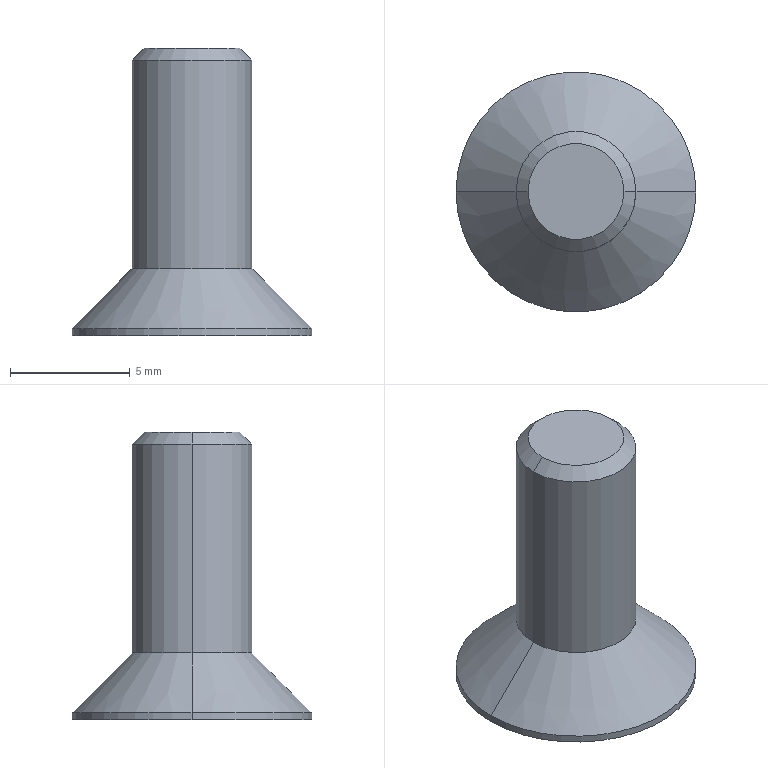Part | SolidWorks | features BaseBody 1 | 1 solid | 24 faces | box 10 x 10 x 12 mm | volume 284.359 mm3 | plane 14 | cone 6 | cylinder 4 | commonest cylinder face diameters 5 x2 10 x2
STEP:
#1=CARTESIAN_POINT('',(-2.5,0.,11.5));
#2=VERTEX_POINT('',#1);
#3=CARTESIAN_POINT('',(2.5,0.,11.5));
#4=VERTEX_POINT('',#3);
#5=CARTESIAN_POINT('',(0.,0.,11.5));
#6=DIRECTION('',(0.,0.,-1.));
#7=DIRECTION('',(-1.,0.,0.));
#8=AXIS2_PLACEMENT_3D('',#5,#6,#7);
#9=CIRCLE('',#8,2.5);
#10=EDGE_CURVE('',#2,#4,#9,.T.);
#11=ORIENTED_EDGE('',*,*,#10,.T.);
#12=CARTESIAN_POINT('',(2.5,0.,2.8));
#13=VERTEX_POINT('',#12);
#14=CARTESIAN_POINT('',(2.5,0.,12.));
#15=DIRECTION('',(0.,0.,-1.));
#16=VECTOR('',#15,1000.);
#17=LINE('',#14,#16);
#18=EDGE_CURVE('',#4,#13,#17,.T.);
#19=ORIENTED_EDGE('',*,*,#18,.T.);
#20=CARTESIAN_POINT('',(-2.5,0.,2.8));
#21=VERTEX_POINT('',#20);
#22=CARTESIAN_POINT('',(0.,0.,2.8));
#23=DIRECTION('',(0.,0.,1.));
#24=DIRECTION('',(-1.,0.,0.));
#25=AXIS2_PLACEMENT_3D('',#22,#23,#24);
#26=CIRCLE('',#25,2.5);
#27=EDGE_CURVE('',#13,#21,#26,.T.);
#28=ORIENTED_EDGE('',*,*,#27,.T.);
#29=CARTESIAN_POINT('',(-2.5,0.,12.));
#30=DIRECTION('',(0.,0.,-1.));
#31=VECTOR('',#30,1000.);
#32=LINE('',#29,#31);
#33=EDGE_CURVE('',#2,#21,#32,.T.);
#34=ORIENTED_EDGE('',*,*,#33,.F.);
#35=EDGE_LOOP('',(#11,#19,#28,#34));
#36=FACE_OUTER_BOUND('',#35,.T.);
#37=CARTESIAN_POINT('',(0.,0.,12.));
#38=DIRECTION('',(0.,0.,-1.));
#39=DIRECTION('',(-1.,0.,0.));
#40=AXIS2_PLACEMENT_3D('',#37,#38,#39);
#41=CYLINDRICAL_SURFACE('',#40,2.5);
#42=ADVANCED_FACE('',(#36),#41,.T.);
#43=ORIENTED_EDGE('',*,*,#27,.F.);
#44=CARTESIAN_POINT('',(5.,0.,0.3));
#45=VERTEX_POINT('',#44);
#46=CARTESIAN_POINT('',(5.,0.,0.3));
#47=DIRECTION('',(0.7071,0.,-0.7071));
#48=VECTOR('',#47,1000.);
#49=LINE('',#46,#48);
#50=EDGE_CURVE('',#13,#45,#49,.T.);
#51=ORIENTED_EDGE('',*,*,#50,.T.);
#52=CARTESIAN_POINT('',(-5.,0.,0.3));
#53=VERTEX_POINT('',#52);
#54=CARTESIAN_POINT('',(0.,0.,0.3));
#55=DIRECTION('',(0.,0.,1.));
#56=DIRECTION('',(-1.,0.,0.));
#57=AXIS2_PLACEMENT_3D('',#54,#55,#56);
#58=CIRCLE('',#57,5.);
#59=EDGE_CURVE('',#45,#53,#58,.T.);
#60=ORIENTED_EDGE('',*,*,#59,.T.);
#61=CARTESIAN_POINT('',(-5.,0.,0.3));
#62=DIRECTION('',(-0.7071,0.,-0.7071));
#63=VECTOR('',#62,1000.);
#64=LINE('',#61,#63);
#65=EDGE_CURVE('',#21,#53,#64,.T.);
#66=ORIENTED_EDGE('',*,*,#65,.F.);
#67=EDGE_LOOP('',(#43,#51,#60,#66));
#68=FACE_OUTER_BOUND('',#67,.T.);
#69=CARTESIAN_POINT('',(0.,0.,0.3));
#70=DIRECTION('',(0.,0.,-1.));
#71=DIRECTION('',(-1.,0.,0.));
#72=AXIS2_PLACEMENT_3D('',#69,#70,#71);
#73=CONICAL_SURFACE('',#72,5.,0.7854);
#74=ADVANCED_FACE('',(#68),#73,.T.);
#75=CARTESIAN_POINT('',(-2.,0.,12.));
#76=VERTEX_POINT('',#75);
#77=CARTESIAN_POINT('',(2.,0.,12.));
#78=VERTEX_POINT('',#77);
#79=CARTESIAN_POINT('',(0.,0.,12.));
#80=DIRECTION('',(0.,0.,-1.));
#81=DIRECTION('',(-1.,0.,0.));
#82=AXIS2_PLACEMENT_3D('',#79,#80,#81);
#83=CIRCLE('',#82,2.);
#84=EDGE_CURVE('',#76,#78,#83,.T.);
#85=ORIENTED_EDGE('',*,*,#84,.T.);
#86=CARTESIAN_POINT('',(2.5,0.,11.5));
#87=DIRECTION('',(0.7071,0.,-0.7071));
#88=VECTOR('',#87,1000.);
#89=LINE('',#86,#88);
#90=EDGE_CURVE('',#78,#4,#89,.T.);
#91=ORIENTED_EDGE('',*,*,#90,.T.);
#92=ORIENTED_EDGE('',*,*,#10,.F.);
#93=CARTESIAN_POINT('',(-2.5,0.,11.5));
#94=DIRECTION('',(-0.7071,0.,-0.7071));
#95=VECTOR('',#94,1000.);
#96=LINE('',#93,#95);
#97=EDGE_CURVE('',#76,#2,#96,.T.);
#98=ORIENTED_EDGE('',*,*,#97,.F.);
#99=EDGE_LOOP('',(#85,#91,#92,#98));
#100=FACE_OUTER_BOUND('',#99,.T.);
#101=CARTESIAN_POINT('',(0.,0.,11.5));
#102=DIRECTION('',(0.,0.,-1.));
#103=DIRECTION('',(-1.,0.,0.));
#104=AXIS2_PLACEMENT_3D('',#101,#102,#103);
#105=CONICAL_SURFACE('',#104,2.5,0.7854);
#106=ADVANCED_FACE('',(#100),#105,.T.);
#107=ORIENTED_EDGE('',*,*,#59,.F.);
#108=CARTESIAN_POINT('',(5.,0.,0.));
#109=VERTEX_POINT('',#108);
#110=CARTESIAN_POINT('',(5.,0.,2.8));
#111=DIRECTION('',(0.,0.,-1.));
#112=VECTOR('',#111,1000.);
#113=LINE('',#110,#112);
#114=EDGE_CURVE('',#45,#109,#113,.T.);
#115=ORIENTED_EDGE('',*,*,#114,.T.);
#116=CARTESIAN_POINT('',(-5.,0.,0.));
#117=VERTEX_POINT('',#116);
#118=CARTESIAN_POINT('',(0.,0.,0.));
#119=DIRECTION('',(0.,0.,1.));
#120=DIRECTION('',(-1.,0.,0.));
#121=AXIS2_PLACEMENT_3D('',#118,#119,#120);
#122=CIRCLE('',#121,5.);
#123=EDGE_CURVE('',#109,#117,#122,.T.);
#124=ORIENTED_EDGE('',*,*,#123,.T.);
#125=CARTESIAN_POINT('',(-5.,0.,2.8));
#126=DIRECTION('',(0.,0.,-1.));
#127=VECTOR('',#126,1000.);
#128=LINE('',#125,#127);
#129=EDGE_CURVE('',#53,#117,#128,.T.);
#130=ORIENTED_EDGE('',*,*,#129,.F.);
#131=EDGE_LOOP('',(#107,#115,#124,#130));
#132=FACE_OUTER_BOUND('',#131,.T.);
#133=CARTESIAN_POINT('',(0.,0.,2.8));
#134=DIRECTION('',(0.,0.,-1.));
#135=DIRECTION('',(-1.,0.,0.));
#136=AXIS2_PLACEMENT_3D('',#133,#134,#135);
#137=CYLINDRICAL_SURFACE('',#136,5.);
#138=ADVANCED_FACE('',(#132),#137,.T.);
#139=CARTESIAN_POINT('',(0.,0.,3.155));
#140=VERTEX_POINT('',#139);
#141=CARTESIAN_POINT('',(-2.,0.,2.));
#142=VERTEX_POINT('',#141);
#143=CARTESIAN_POINT('',(-2.,0.,2.));
#144=DIRECTION('',(-0.866,0.,-0.5));
#145=VECTOR('',#144,1000.);
#146=LINE('',#143,#145);
#147=EDGE_CURVE('',#140,#142,#146,.T.);
#148=ORIENTED_EDGE('',*,*,#147,.F.);
#149=CARTESIAN_POINT('',(2.,0.,2.));
#150=VERTEX_POINT('',#149);
#151=CARTESIAN_POINT('',(2.,0.,2.));
#152=DIRECTION('',(0.866,0.,-0.5));
#153=VECTOR('',#152,1000.);
#154=LINE('',#151,#153);
#155=EDGE_CURVE('',#140,#150,#154,.T.);
#156=ORIENTED_EDGE('',*,*,#155,.T.);
#157=CARTESIAN_POINT('',(1.732,-1.,2.));
#158=VERTEX_POINT('',#157);
#159=CARTESIAN_POINT('',(0.,0.,2.));
#160=DIRECTION('',(0.,0.,1.));
#161=DIRECTION('',(-1.,0.,0.));
#162=AXIS2_PLACEMENT_3D('',#159,#160,#161);
#163=CIRCLE('',#162,2.);
#164=EDGE_CURVE('',#158,#150,#163,.T.);
#165=ORIENTED_EDGE('',*,*,#164,.F.);
#166=CARTESIAN_POINT('',(0.,-2.,2.));
#167=VERTEX_POINT('',#166);
#168=CARTESIAN_POINT('',(0.,0.,2.));
#169=DIRECTION('',(0.,0.,1.));
#170=DIRECTION('',(-1.,0.,0.));
#171=AXIS2_PLACEMENT_3D('',#168,#169,#170);
#172=CIRCLE('',#171,2.);
#173=EDGE_CURVE('',#167,#158,#172,.T.);
#174=ORIENTED_EDGE('',*,*,#173,.F.);
#175=CARTESIAN_POINT('',(-1.732,-1.,2.));
#176=VERTEX_POINT('',#175);
#177=CARTESIAN_POINT('',(0.,0.,2.));
#178=DIRECTION('',(0.,0.,1.));
#179=DIRECTION('',(-1.,0.,0.));
#180=AXIS2_PLACEMENT_3D('',#177,#178,#179);
#181=CIRCLE('',#180,2.);
#182=EDGE_CURVE('',#176,#167,#181,.T.);
#183=ORIENTED_EDGE('',*,*,#182,.F.);
#184=CARTESIAN_POINT('',(0.,0.,2.));
#185=DIRECTION('',(0.,0.,1.));
#186=DIRECTION('',(-1.,0.,0.));
#187=AXIS2_PLACEMENT_3D('',#184,#185,#186);
#188=CIRCLE('',#187,2.);
#189=EDGE_CURVE('',#142,#176,#188,.T.);
#190=ORIENTED_EDGE('',*,*,#189,.F.);
#191=EDGE_LOOP('',(#148,#156,#165,#174,#183,#190));
#192=FACE_OUTER_BOUND('',#191,.T.);
#193=CARTESIAN_POINT('',(0.,0.,2.));
#194=DIRECTION('',(0.,0.,-1.));
#195=DIRECTION('',(-1.,0.,0.));
#196=AXIS2_PLACEMENT_3D('',#193,#194,#195);
#197=CONICAL_SURFACE('',#196,2.,1.047);
#198=ADVANCED_FACE('',(#192),#197,.F.);
#199=ORIENTED_EDGE('',*,*,#18,.F.);
#200=CARTESIAN_POINT('',(0.,0.,11.5));
#201=DIRECTION('',(0.,0.,-1.));
#202=DIRECTION('',(-1.,0.,0.));
#203=AXIS2_PLACEMENT_3D('',#200,#201,#202);
#204=CIRCLE('',#203,2.5);
#205=EDGE_CURVE('',#4,#2,#204,.T.);
#206=ORIENTED_EDGE('',*,*,#205,.T.);
#207=ORIENTED_EDGE('',*,*,#33,.T.);
#208=CARTESIAN_POINT('',(0.,0.,2.8));
#209=DIRECTION('',(0.,0.,1.));
#210=DIRECTION('',(-1.,0.,0.));
#211=AXIS2_PLACEMENT_3D('',#208,#209,#210);
#212=CIRCLE('',#211,2.5);
#213=EDGE_CURVE('',#21,#13,#212,.T.);
#214=ORIENTED_EDGE('',*,*,#213,.T.);
#215=EDGE_LOOP('',(#199,#206,#207,#214));
#216=FACE_OUTER_BOUND('',#215,.T.);
#217=CARTESIAN_POINT('',(0.,0.,12.));
#218=DIRECTION('',(0.,0.,-1.));
#219=DIRECTION('',(-1.,0.,0.));
#220=AXIS2_PLACEMENT_3D('',#217,#218,#219);
#221=CYLINDRICAL_SURFACE('',#220,2.5);
#222=ADVANCED_FACE('',(#216),#221,.T.);
#223=ORIENTED_EDGE('',*,*,#50,.F.);
#224=ORIENTED_EDGE('',*,*,#213,.F.);
#225=ORIENTED_EDGE('',*,*,#65,.T.);
#226=CARTESIAN_POINT('',(0.,0.,0.3));
#227=DIRECTION('',(0.,0.,1.));
#228=DIRECTION('',(-1.,0.,0.));
#229=AXIS2_PLACEMENT_3D('',#226,#227,#228);
#230=CIRCLE('',#229,5.);
#231=EDGE_CURVE('',#53,#45,#230,.T.);
#232=ORIENTED_EDGE('',*,*,#231,.T.);
#233=EDGE_LOOP('',(#223,#224,#225,#232));
#234=FACE_OUTER_BOUND('',#233,.T.);
#235=CARTESIAN_POINT('',(0.,0.,0.3));
#236=DIRECTION('',(0.,0.,-1.));
#237=DIRECTION('',(-1.,0.,0.));
#238=AXIS2_PLACEMENT_3D('',#235,#236,#237);
#239=CONICAL_SURFACE('',#238,5.,0.7854);
#240=ADVANCED_FACE('',(#234),#239,.T.);
#241=ORIENTED_EDGE('',*,*,#90,.F.);
#242=CARTESIAN_POINT('',(0.,0.,12.));
#243=DIRECTION('',(0.,0.,-1.));
#244=DIRECTION('',(-1.,0.,0.));
#245=AXIS2_PLACEMENT_3D('',#242,#243,#244);
#246=CIRCLE('',#245,2.);
#247=EDGE_CURVE('',#78,#76,#246,.T.);
#248=ORIENTED_EDGE('',*,*,#247,.T.);
#249=ORIENTED_EDGE('',*,*,#97,.T.);
#250=ORIENTED_EDGE('',*,*,#205,.F.);
#251=EDGE_LOOP('',(#241,#248,#249,#250));
#252=FACE_OUTER_BOUND('',#251,.T.);
#253=CARTESIAN_POINT('',(0.,0.,11.5));
#254=DIRECTION('',(0.,0.,-1.));
#255=DIRECTION('',(-1.,0.,0.));
#256=AXIS2_PLACEMENT_3D('',#253,#254,#255);
#257=CONICAL_SURFACE('',#256,2.5,0.7854);
#258=ADVANCED_FACE('',(#252),#257,.T.);
#259=ORIENTED_EDGE('',*,*,#114,.F.);
#260=ORIENTED_EDGE('',*,*,#231,.F.);
#261=ORIENTED_EDGE('',*,*,#129,.T.);
#262=CARTESIAN_POINT('',(0.,0.,0.));
#263=DIRECTION('',(0.,0.,1.));
#264=DIRECTION('',(-1.,0.,0.));
#265=AXIS2_PLACEMENT_3D('',#262,#263,#264);
#266=CIRCLE('',#265,5.);
#267=EDGE_CURVE('',#117,#109,#266,.T.);
#268=ORIENTED_EDGE('',*,*,#267,.T.);
#269=EDGE_LOOP('',(#259,#260,#261,#268));
#270=FACE_OUTER_BOUND('',#269,.T.);
#271=CARTESIAN_POINT('',(0.,0.,2.8));
#272=DIRECTION('',(0.,0.,-1.));
#273=DIRECTION('',(-1.,0.,0.));
#274=AXIS2_PLACEMENT_3D('',#271,#272,#273);
#275=CYLINDRICAL_SURFACE('',#274,5.);
#276=ADVANCED_FACE('',(#270),#275,.T.);
#277=ORIENTED_EDGE('',*,*,#84,.F.);
#278=ORIENTED_EDGE('',*,*,#247,.F.);
#279=EDGE_LOOP('',(#277,#278));
#280=FACE_OUTER_BOUND('',#279,.T.);
#281=CARTESIAN_POINT('',(0.,0.,12.));
#282=DIRECTION('',(0.,0.,1.));
#283=DIRECTION('',(1.,0.,0.));
#284=AXIS2_PLACEMENT_3D('',#281,#282,#283);
#285=PLANE('',#284);
#286=ADVANCED_FACE('',(#280),#285,.T.);
#287=ORIENTED_EDGE('',*,*,#267,.F.);
#288=ORIENTED_EDGE('',*,*,#123,.F.);
#289=EDGE_LOOP('',(#287,#288));
#290=FACE_OUTER_BOUND('',#289,.T.);
#291=CARTESIAN_POINT('',(-2.309,0.,0.));
#292=VERTEX_POINT('',#291);
#293=CARTESIAN_POINT('',(-1.155,2.,0.));
#294=VERTEX_POINT('',#293);
#295=CARTESIAN_POINT('',(-2.309,0.,0.));
#296=DIRECTION('',(0.5,0.866,0.));
#297=VECTOR('',#296,1000.);
#298=LINE('',#295,#297);
#299=EDGE_CURVE('',#292,#294,#298,.T.);
#300=ORIENTED_EDGE('',*,*,#299,.F.);
#301=CARTESIAN_POINT('',(-1.155,-2.,0.));
#302=VERTEX_POINT('',#301);
#303=CARTESIAN_POINT('',(-1.155,-2.,0.));
#304=DIRECTION('',(-0.5,0.866,0.));
#305=VECTOR('',#304,1000.);
#306=LINE('',#303,#305);
#307=EDGE_CURVE('',#302,#292,#306,.T.);
#308=ORIENTED_EDGE('',*,*,#307,.F.);
#309=CARTESIAN_POINT('',(1.155,-2.,0.));
#310=VERTEX_POINT('',#309);
#311=CARTESIAN_POINT('',(0.,-2.,0.));
#312=DIRECTION('',(-1.,0.,0.));
#313=VECTOR('',#312,1000.);
#314=LINE('',#311,#313);
#315=EDGE_CURVE('',#310,#302,#314,.T.);
#316=ORIENTED_EDGE('',*,*,#315,.F.);
#317=CARTESIAN_POINT('',(2.309,0.,0.));
#318=VERTEX_POINT('',#317);
#319=CARTESIAN_POINT('',(2.309,0.,0.));
#320=DIRECTION('',(-0.5,-0.866,0.));
#321=VECTOR('',#320,1000.);
#322=LINE('',#319,#321);
#323=EDGE_CURVE('',#318,#310,#322,.T.);
#324=ORIENTED_EDGE('',*,*,#323,.F.);
#325=CARTESIAN_POINT('',(1.155,2.,0.));
#326=VERTEX_POINT('',#325);
#327=CARTESIAN_POINT('',(1.155,2.,0.));
#328=DIRECTION('',(0.5,-0.866,0.));
#329=VECTOR('',#328,1000.);
#330=LINE('',#327,#329);
#331=EDGE_CURVE('',#326,#318,#330,.T.);
#332=ORIENTED_EDGE('',*,*,#331,.F.);
#333=CARTESIAN_POINT('',(0.,2.,0.));
#334=DIRECTION('',(1.,0.,0.));
#335=VECTOR('',#334,1000.);
#336=LINE('',#333,#335);
#337=EDGE_CURVE('',#294,#326,#336,.T.);
#338=ORIENTED_EDGE('',*,*,#337,.F.);
#339=EDGE_LOOP('',(#300,#308,#316,#324,#332,#338));
#340=FACE_BOUND('',#339,.T.);
#341=CARTESIAN_POINT('',(0.,0.,0.));
#342=DIRECTION('',(0.,0.,1.));
#343=DIRECTION('',(1.,0.,0.));
#344=AXIS2_PLACEMENT_3D('',#341,#342,#343);
#345=PLANE('',#344);
#346=ADVANCED_FACE('',(#290,#340),#345,.F.);
#347=CARTESIAN_POINT('',(1.155,2.,2.));
#348=VERTEX_POINT('',#347);
#349=CARTESIAN_POINT('',(1.155,2.,2.));
#350=DIRECTION('',(0.,0.,-1.));
#351=VECTOR('',#350,1000.);
#352=LINE('',#349,#351);
#353=EDGE_CURVE('',#348,#326,#352,.T.);
#354=ORIENTED_EDGE('',*,*,#353,.F.);
#355=CARTESIAN_POINT('',(0.,2.,2.));
#356=VERTEX_POINT('',#355);
#357=CARTESIAN_POINT('',(0.,2.,2.));
#358=DIRECTION('',(1.,0.,0.));
#359=VECTOR('',#358,1000.);
#360=LINE('',#357,#359);
#361=EDGE_CURVE('',#356,#348,#360,.T.);
#362=ORIENTED_EDGE('',*,*,#361,.F.);
#363=CARTESIAN_POINT('',(-1.155,2.,2.));
#364=VERTEX_POINT('',#363);
#365=CARTESIAN_POINT('',(0.,2.,2.));
#366=DIRECTION('',(1.,0.,0.));
#367=VECTOR('',#366,1000.);
#368=LINE('',#365,#367);
#369=EDGE_CURVE('',#364,#356,#368,.T.);
#370=ORIENTED_EDGE('',*,*,#369,.F.);
#371=CARTESIAN_POINT('',(-1.155,2.,2.));
#372=DIRECTION('',(0.,0.,1.));
#373=VECTOR('',#372,1000.);
#374=LINE('',#371,#373);
#375=EDGE_CURVE('',#294,#364,#374,.T.);
#376=ORIENTED_EDGE('',*,*,#375,.F.);
#377=ORIENTED_EDGE('',*,*,#337,.T.);
#378=EDGE_LOOP('',(#354,#362,#370,#376,#377));
#379=FACE_OUTER_BOUND('',#378,.T.);
#380=CARTESIAN_POINT('',(-1.155,2.,2.));
#381=DIRECTION('',(0.,1.,0.));
#382=DIRECTION('',(0.,0.,1.));
#383=AXIS2_PLACEMENT_3D('',#380,#381,#382);
#384=PLANE('',#383);
#385=ADVANCED_FACE('',(#379),#384,.F.);
#386=ORIENTED_EDGE('',*,*,#375,.T.);
#387=CARTESIAN_POINT('',(-1.732,1.,2.));
#388=VERTEX_POINT('',#387);
#389=CARTESIAN_POINT('',(-1.732,1.,2.));
#390=DIRECTION('',(0.5,0.866,0.));
#391=VECTOR('',#390,1000.);
#392=LINE('',#389,#391);
#393=EDGE_CURVE('',#388,#364,#392,.T.);
#394=ORIENTED_EDGE('',*,*,#393,.F.);
#395=CARTESIAN_POINT('',(-2.309,0.,2.));
#396=VERTEX_POINT('',#395);
#397=CARTESIAN_POINT('',(-2.309,0.,2.));
#398=DIRECTION('',(0.5,0.866,0.));
#399=VECTOR('',#398,1000.);
#400=LINE('',#397,#399);
#401=EDGE_CURVE('',#396,#388,#400,.T.);
#402=ORIENTED_EDGE('',*,*,#401,.F.);
#403=CARTESIAN_POINT('',(-2.309,0.,2.));
#404=DIRECTION('',(0.,0.,1.));
#405=VECTOR('',#404,1000.);
#406=LINE('',#403,#405);
#407=EDGE_CURVE('',#292,#396,#406,.T.);
#408=ORIENTED_EDGE('',*,*,#407,.F.);
#409=ORIENTED_EDGE('',*,*,#299,.T.);
#410=EDGE_LOOP('',(#386,#394,#402,#408,#409));
#411=FACE_OUTER_BOUND('',#410,.T.);
#412=CARTESIAN_POINT('',(-2.309,0.,2.));
#413=DIRECTION('',(-0.866,0.5,0.));
#414=DIRECTION('',(-0.5,-0.866,0.));
#415=AXIS2_PLACEMENT_3D('',#412,#413,#414);
#416=PLANE('',#415);
#417=ADVANCED_FACE('',(#411),#416,.F.);
#418=ORIENTED_EDGE('',*,*,#407,.T.);
#419=CARTESIAN_POINT('',(-1.155,-2.,2.));
#420=DIRECTION('',(-0.5,0.866,0.));
#421=VECTOR('',#420,1000.);
#422=LINE('',#419,#421);
#423=EDGE_CURVE('',#176,#396,#422,.T.);
#424=ORIENTED_EDGE('',*,*,#423,.F.);
#425=CARTESIAN_POINT('',(-1.155,-2.,2.));
#426=VERTEX_POINT('',#425);
#427=CARTESIAN_POINT('',(-1.155,-2.,2.));
#428=DIRECTION('',(-0.5,0.866,0.));
#429=VECTOR('',#428,1000.);
#430=LINE('',#427,#429);
#431=EDGE_CURVE('',#426,#176,#430,.T.);
#432=ORIENTED_EDGE('',*,*,#431,.F.);
#433=CARTESIAN_POINT('',(-1.155,-2.,2.));
#434=DIRECTION('',(0.,0.,1.));
#435=VECTOR('',#434,1000.);
#436=LINE('',#433,#435);
#437=EDGE_CURVE('',#302,#426,#436,.T.);
#438=ORIENTED_EDGE('',*,*,#437,.F.);
#439=ORIENTED_EDGE('',*,*,#307,.T.);
#440=EDGE_LOOP('',(#418,#424,#432,#438,#439));
#441=FACE_OUTER_BOUND('',#440,.T.);
#442=CARTESIAN_POINT('',(-1.155,-2.,2.));
#443=DIRECTION('',(-0.866,-0.5,0.));
#444=DIRECTION('',(0.5,-0.866,0.));
#445=AXIS2_PLACEMENT_3D('',#442,#443,#444);
#446=PLANE('',#445);
#447=ADVANCED_FACE('',(#441),#446,.F.);
#448=ORIENTED_EDGE('',*,*,#437,.T.);
#449=CARTESIAN_POINT('',(0.,-2.,2.));
#450=DIRECTION('',(-1.,0.,0.));
#451=VECTOR('',#450,1000.);
#452=LINE('',#449,#451);
#453=EDGE_CURVE('',#167,#426,#452,.T.);
#454=ORIENTED_EDGE('',*,*,#453,.F.);
#455=CARTESIAN_POINT('',(1.155,-2.,2.));
#456=VERTEX_POINT('',#455);
#457=CARTESIAN_POINT('',(0.,-2.,2.));
#458=DIRECTION('',(-1.,0.,0.));
#459=VECTOR('',#458,1000.);
#460=LINE('',#457,#459);
#461=EDGE_CURVE('',#456,#167,#460,.T.);
#462=ORIENTED_EDGE('',*,*,#461,.F.);
#463=CARTESIAN_POINT('',(1.155,-2.,2.));
#464=DIRECTION('',(0.,0.,1.));
#465=VECTOR('',#464,1000.);
#466=LINE('',#463,#465);
#467=EDGE_CURVE('',#310,#456,#466,.T.);
#468=ORIENTED_EDGE('',*,*,#467,.F.);
#469=ORIENTED_EDGE('',*,*,#315,.T.);
#470=EDGE_LOOP('',(#448,#454,#462,#468,#469));
#471=FACE_OUTER_BOUND('',#470,.T.);
#472=CARTESIAN_POINT('',(1.155,-2.,2.));
#473=DIRECTION('',(0.,-1.,0.));
#474=DIRECTION('',(1.,0.,0.));
#475=AXIS2_PLACEMENT_3D('',#472,#473,#474);
#476=PLANE('',#475);
#477=ADVANCED_FACE('',(#471),#476,.F.);
#478=ORIENTED_EDGE('',*,*,#467,.T.);
#479=CARTESIAN_POINT('',(1.732,-1.,2.));
#480=DIRECTION('',(-0.5,-0.866,0.));
#481=VECTOR('',#480,1000.);
#482=LINE('',#479,#481);
#483=EDGE_CURVE('',#158,#456,#482,.T.);
#484=ORIENTED_EDGE('',*,*,#483,.F.);
#485=CARTESIAN_POINT('',(2.309,0.,2.));
#486=VERTEX_POINT('',#485);
#487=CARTESIAN_POINT('',(2.309,0.,2.));
#488=DIRECTION('',(-0.5,-0.866,0.));
#489=VECTOR('',#488,1000.);
#490=LINE('',#487,#489);
#491=EDGE_CURVE('',#486,#158,#490,.T.);
#492=ORIENTED_EDGE('',*,*,#491,.F.);
#493=CARTESIAN_POINT('',(2.309,0.,2.));
#494=DIRECTION('',(0.,0.,1.));
#495=VECTOR('',#494,1000.);
#496=LINE('',#493,#495);
#497=EDGE_CURVE('',#318,#486,#496,.T.);
#498=ORIENTED_EDGE('',*,*,#497,.F.);
#499=ORIENTED_EDGE('',*,*,#323,.T.);
#500=EDGE_LOOP('',(#478,#484,#492,#498,#499));
#501=FACE_OUTER_BOUND('',#500,.T.);
#502=CARTESIAN_POINT('',(2.309,0.,2.));
#503=DIRECTION('',(0.866,-0.5,0.));
#504=DIRECTION('',(0.5,0.866,0.));
#505=AXIS2_PLACEMENT_3D('',#502,#503,#504);
#506=PLANE('',#505);
#507=ADVANCED_FACE('',(#501),#506,.F.);
#508=ORIENTED_EDGE('',*,*,#497,.T.);
#509=CARTESIAN_POINT('',(1.732,1.,2.));
#510=VERTEX_POINT('',#509);
#511=CARTESIAN_POINT('',(1.155,2.,2.));
#512=DIRECTION('',(0.5,-0.866,0.));
#513=VECTOR('',#512,1000.);
#514=LINE('',#511,#513);
#515=EDGE_CURVE('',#510,#486,#514,.T.);
#516=ORIENTED_EDGE('',*,*,#515,.F.);
#517=CARTESIAN_POINT('',(1.155,2.,2.));
#518=DIRECTION('',(0.5,-0.866,0.));
#519=VECTOR('',#518,1000.);
#520=LINE('',#517,#519);
#521=EDGE_CURVE('',#348,#510,#520,.T.);
#522=ORIENTED_EDGE('',*,*,#521,.F.);
#523=ORIENTED_EDGE('',*,*,#353,.T.);
#524=ORIENTED_EDGE('',*,*,#331,.T.);
#525=EDGE_LOOP('',(#508,#516,#522,#523,#524));
#526=FACE_OUTER_BOUND('',#525,.T.);
#527=CARTESIAN_POINT('',(1.155,2.,2.));
#528=DIRECTION('',(0.866,0.5,0.));
#529=DIRECTION('',(-0.5,0.866,0.));
#530=AXIS2_PLACEMENT_3D('',#527,#528,#529);
#531=PLANE('',#530);
#532=ADVANCED_FACE('',(#526),#531,.F.);
#533=ORIENTED_EDGE('',*,*,#401,.T.);
#534=CARTESIAN_POINT('',(0.,0.,2.));
#535=DIRECTION('',(0.,0.,1.));
#536=DIRECTION('',(-1.,0.,0.));
#537=AXIS2_PLACEMENT_3D('',#534,#535,#536);
#538=CIRCLE('',#537,2.);
#539=EDGE_CURVE('',#388,#142,#538,.T.);
#540=ORIENTED_EDGE('',*,*,#539,.T.);
#541=ORIENTED_EDGE('',*,*,#189,.T.);
#542=ORIENTED_EDGE('',*,*,#423,.T.);
#543=EDGE_LOOP('',(#533,#540,#541,#542));
#544=FACE_OUTER_BOUND('',#543,.T.);
#545=CARTESIAN_POINT('',(0.,0.,2.));
#546=DIRECTION('',(0.,0.,-1.));
#547=DIRECTION('',(-1.,0.,0.));
#548=AXIS2_PLACEMENT_3D('',#545,#546,#547);
#549=PLANE('',#548);
#550=ADVANCED_FACE('',(#544),#549,.T.);
#551=ORIENTED_EDGE('',*,*,#491,.T.);
#552=ORIENTED_EDGE('',*,*,#164,.T.);
#553=CARTESIAN_POINT('',(0.,0.,2.));
#554=DIRECTION('',(0.,0.,1.));
#555=DIRECTION('',(-1.,0.,0.));
#556=AXIS2_PLACEMENT_3D('',#553,#554,#555);
#557=CIRCLE('',#556,2.);
#558=EDGE_CURVE('',#150,#510,#557,.T.);
#559=ORIENTED_EDGE('',*,*,#558,.T.);
#560=ORIENTED_EDGE('',*,*,#515,.T.);
#561=EDGE_LOOP('',(#551,#552,#559,#560));
#562=FACE_OUTER_BOUND('',#561,.T.);
#563=CARTESIAN_POINT('',(0.,0.,2.));
#564=DIRECTION('',(0.,0.,-1.));
#565=DIRECTION('',(-1.,0.,0.));
#566=AXIS2_PLACEMENT_3D('',#563,#564,#565);
#567=PLANE('',#566);
#568=ADVANCED_FACE('',(#562),#567,.T.);
#569=ORIENTED_EDGE('',*,*,#361,.T.);
#570=ORIENTED_EDGE('',*,*,#521,.T.);
#571=CARTESIAN_POINT('',(0.,0.,2.));
#572=DIRECTION('',(0.,0.,1.));
#573=DIRECTION('',(-1.,0.,0.));
#574=AXIS2_PLACEMENT_3D('',#571,#572,#573);
#575=CIRCLE('',#574,2.);
#576=EDGE_CURVE('',#510,#356,#575,.T.);
#577=ORIENTED_EDGE('',*,*,#576,.T.);
#578=EDGE_LOOP('',(#569,#570,#577));
#579=FACE_OUTER_BOUND('',#578,.T.);
#580=CARTESIAN_POINT('',(0.,0.,2.));
#581=DIRECTION('',(0.,0.,-1.));
#582=DIRECTION('',(-1.,0.,0.));
#583=AXIS2_PLACEMENT_3D('',#580,#581,#582);
#584=PLANE('',#583);
#585=ADVANCED_FACE('',(#579),#584,.T.);
#586=ORIENTED_EDGE('',*,*,#155,.F.);
#587=ORIENTED_EDGE('',*,*,#147,.T.);
#588=ORIENTED_EDGE('',*,*,#539,.F.);
#589=CARTESIAN_POINT('',(0.,0.,2.));
#590=DIRECTION('',(0.,0.,1.));
#591=DIRECTION('',(-1.,0.,0.));
#592=AXIS2_PLACEMENT_3D('',#589,#590,#591);
#593=CIRCLE('',#592,2.);
#594=EDGE_CURVE('',#356,#388,#593,.T.);
#595=ORIENTED_EDGE('',*,*,#594,.F.);
#596=ORIENTED_EDGE('',*,*,#576,.F.);
#597=ORIENTED_EDGE('',*,*,#558,.F.);
#598=EDGE_LOOP('',(#586,#587,#588,#595,#596,#597));
#599=FACE_OUTER_BOUND('',#598,.T.);
#600=CARTESIAN_POINT('',(0.,0.,2.));
#601=DIRECTION('',(0.,0.,-1.));
#602=DIRECTION('',(-1.,0.,0.));
#603=AXIS2_PLACEMENT_3D('',#600,#601,#602);
#604=CONICAL_SURFACE('',#603,2.,1.047);
#605=ADVANCED_FACE('',(#599),#604,.F.);
#606=ORIENTED_EDGE('',*,*,#393,.T.);
#607=ORIENTED_EDGE('',*,*,#369,.T.);
#608=ORIENTED_EDGE('',*,*,#594,.T.);
#609=EDGE_LOOP('',(#606,#607,#608));
#610=FACE_OUTER_BOUND('',#609,.T.);
#611=CARTESIAN_POINT('',(0.,0.,2.));
#612=DIRECTION('',(0.,0.,-1.));
#613=DIRECTION('',(-1.,0.,0.));
#614=AXIS2_PLACEMENT_3D('',#611,#612,#613);
#615=PLANE('',#614);
#616=ADVANCED_FACE('',(#610),#615,.T.);
#617=ORIENTED_EDGE('',*,*,#483,.T.);
#618=ORIENTED_EDGE('',*,*,#461,.T.);
#619=ORIENTED_EDGE('',*,*,#173,.T.);
#620=EDGE_LOOP('',(#617,#618,#619));
#621=FACE_OUTER_BOUND('',#620,.T.);
#622=CARTESIAN_POINT('',(0.,0.,2.));
#623=DIRECTION('',(0.,0.,-1.));
#624=DIRECTION('',(-1.,0.,0.));
#625=AXIS2_PLACEMENT_3D('',#622,#623,#624);
#626=PLANE('',#625);
#627=ADVANCED_FACE('',(#621),#626,.T.);
#628=ORIENTED_EDGE('',*,*,#453,.T.);
#629=ORIENTED_EDGE('',*,*,#431,.T.);
#630=ORIENTED_EDGE('',*,*,#182,.T.);
#631=EDGE_LOOP('',(#628,#629,#630));
#632=FACE_OUTER_BOUND('',#631,.T.);
#633=CARTESIAN_POINT('',(0.,0.,2.));
#634=DIRECTION('',(0.,0.,-1.));
#635=DIRECTION('',(-1.,0.,0.));
#636=AXIS2_PLACEMENT_3D('',#633,#634,#635);
#637=PLANE('',#636);
#638=ADVANCED_FACE('',(#632),#637,.T.);
#639=CLOSED_SHELL('',(#42,#74,#106,#138,#198,#222,#240,#258,#276,#286,#346,#385,#417,#447,#477,#507,#532,#550,#568,#585,#605,#616,#627,#638));
#640=MANIFOLD_SOLID_BREP('',#639);
#641=CARTESIAN_POINT('',(0.,0.,0.));
#642=DIRECTION('',(0.,0.,1.));
#643=DIRECTION('',(1.,0.,0.));
#644=AXIS2_PLACEMENT_3D('',#641,#642,#643);
#645=(LENGTH_UNIT()NAMED_UNIT(*)SI_UNIT(.MILLI.,.METRE.));
#646=UNCERTAINTY_MEASURE_WITH_UNIT(LENGTH_MEASURE(0.00001),#645,'','');
#647=(NAMED_UNIT(*)PLANE_ANGLE_UNIT()SI_UNIT($,.RADIAN.));
#648=(NAMED_UNIT(*)SI_UNIT($,.STERADIAN.)SOLID_ANGLE_UNIT());
#649=(GEOMETRIC_REPRESENTATION_CONTEXT(3)GLOBAL_UNCERTAINTY_ASSIGNED_CONTEXT((#646))GLOBAL_UNIT_ASSIGNED_CONTEXT((#645,#647,#648))REPRESENTATION_CONTEXT('',''));
#650=ADVANCED_BREP_SHAPE_REPRESENTATION('',(#640,#644),#649);